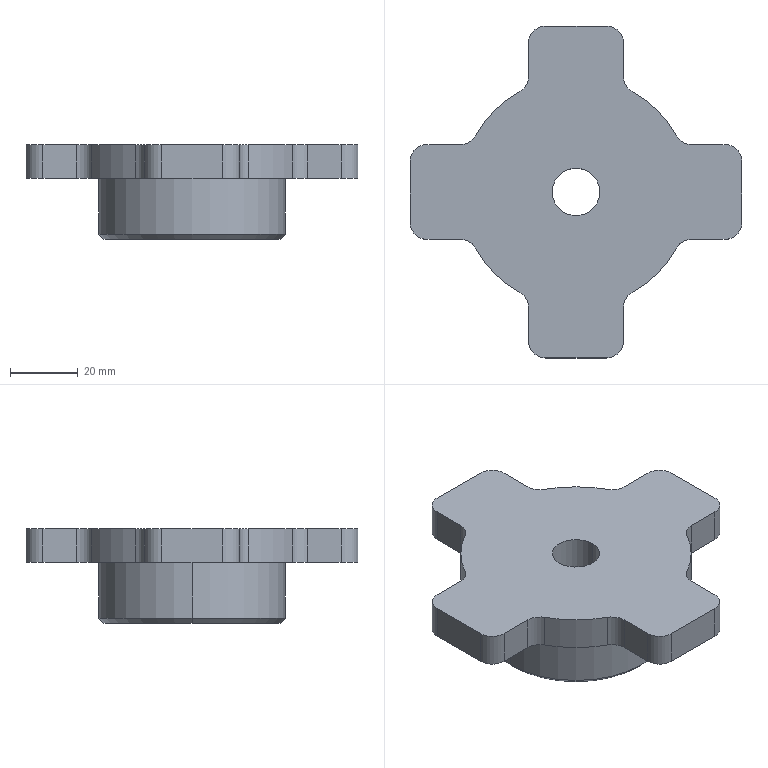Part | STEP file | Foot adjusting disc | 1 solid | 44 faces | box 97.968 x 97.968 x 28 mm | volume 66304 mm3 | cylinder 26 | plane 16 | cone 2 | commonest cylinder face diameters 10 x16 68 x4 14 x2 45 x2 55 x2